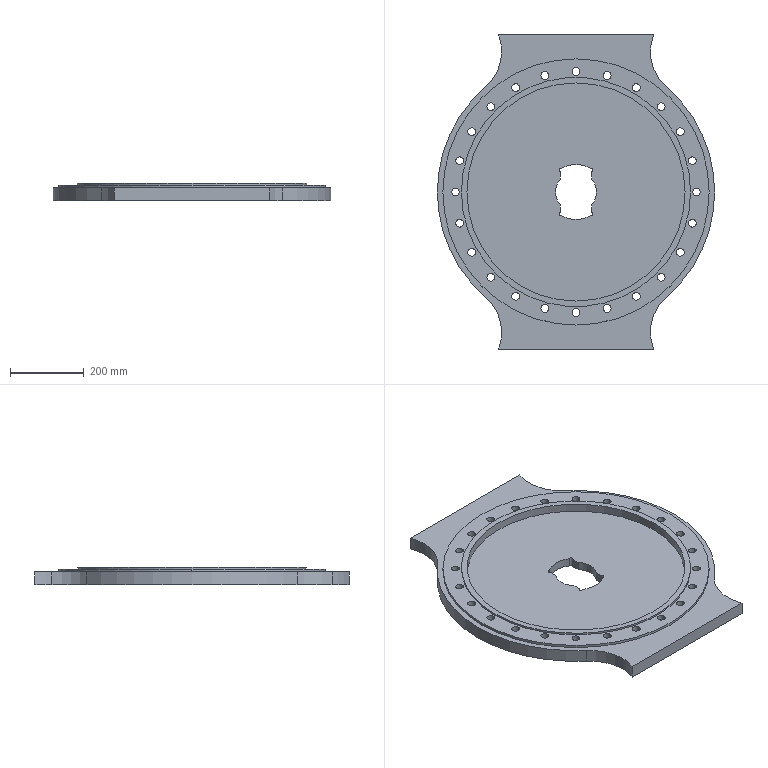Part | SolidWorks | features ICE 4, BaseBody 1 | 1 solid | 85 faces | box 750 x 850 x 47 mm | volume 14896287 mm3 | cylinder 74 | plane 11 | commonest cylinder face diameters 21 x48 10 x6 250 x6 110.5 x3 750 x3 149.5 x2